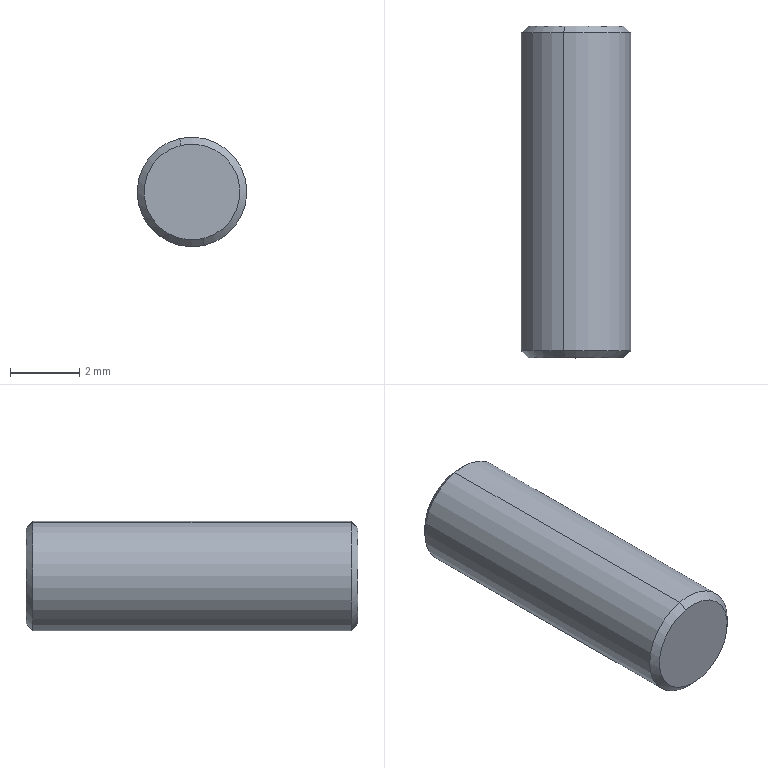Part | STEP file | 4-20.sldasm-Part-227 | 1 solid | 8 faces | box 3.175 x 9.6 x 3.175 mm | volume 75.624 mm3 | cone 4 | cylinder 2 | plane 2 | commonest cylinder face diameters 3.175 x2
STEP:
#1=CARTESIAN_POINT('',(146.186,602.225,-119.7));
#2=VERTEX_POINT('',#1);
#3=CARTESIAN_POINT('',(145.562,602.225,-116.996));
#4=VERTEX_POINT('',#3);
#5=CARTESIAN_POINT('',(145.874,602.225,-118.348));
#6=DIRECTION('',(0.,-1.,0.));
#7=DIRECTION('',(-0.225,0.,0.9744));
#8=AXIS2_PLACEMENT_3D('',#5,#6,#7);
#9=CIRCLE('',#8,1.387);
#10=EDGE_CURVE('',#2,#4,#9,.T.);
#11=ORIENTED_EDGE('',*,*,#10,.T.);
#12=CARTESIAN_POINT('',(145.517,602.025,-116.801));
#13=VERTEX_POINT('',#12);
#14=CARTESIAN_POINT('',(145.562,602.225,-116.996));
#15=DIRECTION('',(-0.1591,-0.7071,0.689));
#16=VECTOR('',#15,1000.);
#17=LINE('',#14,#16);
#18=EDGE_CURVE('',#4,#13,#17,.T.);
#19=ORIENTED_EDGE('',*,*,#18,.T.);
#20=CARTESIAN_POINT('',(146.231,602.025,-119.895));
#21=VERTEX_POINT('',#20);
#22=CARTESIAN_POINT('',(145.874,602.025,-118.348));
#23=DIRECTION('',(0.,1.,0.));
#24=DIRECTION('',(-0.225,0.,0.9744));
#25=AXIS2_PLACEMENT_3D('',#22,#23,#24);
#26=CIRCLE('',#25,1.587);
#27=EDGE_CURVE('',#13,#21,#26,.T.);
#28=ORIENTED_EDGE('',*,*,#27,.T.);
#29=CARTESIAN_POINT('',(146.186,602.225,-119.7));
#30=DIRECTION('',(0.1591,-0.7071,-0.689));
#31=VECTOR('',#30,1000.);
#32=LINE('',#29,#31);
#33=EDGE_CURVE('',#2,#21,#32,.T.);
#34=ORIENTED_EDGE('',*,*,#33,.F.);
#35=EDGE_LOOP('',(#11,#19,#28,#34));
#36=FACE_OUTER_BOUND('',#35,.T.);
#37=CARTESIAN_POINT('',(145.874,602.225,-118.348));
#38=DIRECTION('',(0.,-1.,0.));
#39=DIRECTION('',(0.225,0.,-0.9744));
#40=AXIS2_PLACEMENT_3D('',#37,#38,#39);
#41=CONICAL_SURFACE('',#40,1.387,0.7854);
#42=ADVANCED_FACE('',(#36),#41,.T.);
#43=CARTESIAN_POINT('',(145.562,592.625,-116.996));
#44=VERTEX_POINT('',#43);
#45=CARTESIAN_POINT('',(146.186,592.625,-119.7));
#46=VERTEX_POINT('',#45);
#47=CARTESIAN_POINT('',(145.874,592.625,-118.348));
#48=DIRECTION('',(0.,1.,0.));
#49=DIRECTION('',(-0.225,0.,0.9744));
#50=AXIS2_PLACEMENT_3D('',#47,#48,#49);
#51=CIRCLE('',#50,1.387);
#52=EDGE_CURVE('',#44,#46,#51,.T.);
#53=ORIENTED_EDGE('',*,*,#52,.T.);
#54=CARTESIAN_POINT('',(146.231,592.825,-119.895));
#55=VERTEX_POINT('',#54);
#56=CARTESIAN_POINT('',(146.231,592.825,-119.895));
#57=DIRECTION('',(0.1591,0.7071,-0.689));
#58=VECTOR('',#57,1000.);
#59=LINE('',#56,#58);
#60=EDGE_CURVE('',#46,#55,#59,.T.);
#61=ORIENTED_EDGE('',*,*,#60,.T.);
#62=CARTESIAN_POINT('',(145.517,592.825,-116.801));
#63=VERTEX_POINT('',#62);
#64=CARTESIAN_POINT('',(145.874,592.825,-118.348));
#65=DIRECTION('',(0.,-1.,0.));
#66=DIRECTION('',(-0.225,0.,0.9744));
#67=AXIS2_PLACEMENT_3D('',#64,#65,#66);
#68=CIRCLE('',#67,1.587);
#69=EDGE_CURVE('',#55,#63,#68,.T.);
#70=ORIENTED_EDGE('',*,*,#69,.T.);
#71=CARTESIAN_POINT('',(145.517,592.825,-116.801));
#72=DIRECTION('',(-0.1591,0.7071,0.689));
#73=VECTOR('',#72,1000.);
#74=LINE('',#71,#73);
#75=EDGE_CURVE('',#44,#63,#74,.T.);
#76=ORIENTED_EDGE('',*,*,#75,.F.);
#77=EDGE_LOOP('',(#53,#61,#70,#76));
#78=FACE_OUTER_BOUND('',#77,.T.);
#79=CARTESIAN_POINT('',(145.874,592.825,-118.348));
#80=DIRECTION('',(0.,1.,0.));
#81=DIRECTION('',(-0.225,0.,0.9744));
#82=AXIS2_PLACEMENT_3D('',#79,#80,#81);
#83=CONICAL_SURFACE('',#82,1.587,0.7854);
#84=ADVANCED_FACE('',(#78),#83,.T.);
#85=ORIENTED_EDGE('',*,*,#27,.F.);
#86=CARTESIAN_POINT('',(145.517,602.425,-116.801));
#87=DIRECTION('',(0.,-1.,0.));
#88=VECTOR('',#87,1000.);
#89=LINE('',#86,#88);
#90=EDGE_CURVE('',#13,#63,#89,.T.);
#91=ORIENTED_EDGE('',*,*,#90,.T.);
#92=ORIENTED_EDGE('',*,*,#69,.F.);
#93=CARTESIAN_POINT('',(146.231,602.425,-119.895));
#94=DIRECTION('',(0.,-1.,0.));
#95=VECTOR('',#94,1000.);
#96=LINE('',#93,#95);
#97=EDGE_CURVE('',#21,#55,#96,.T.);
#98=ORIENTED_EDGE('',*,*,#97,.F.);
#99=EDGE_LOOP('',(#85,#91,#92,#98));
#100=FACE_OUTER_BOUND('',#99,.T.);
#101=CARTESIAN_POINT('',(145.874,602.425,-118.348));
#102=DIRECTION('',(0.,-1.,0.));
#103=DIRECTION('',(0.225,0.,-0.9744));
#104=AXIS2_PLACEMENT_3D('',#101,#102,#103);
#105=CYLINDRICAL_SURFACE('',#104,1.587);
#106=ADVANCED_FACE('',(#100),#105,.T.);
#107=ORIENTED_EDGE('',*,*,#90,.F.);
#108=CARTESIAN_POINT('',(145.874,602.025,-118.348));
#109=DIRECTION('',(0.,1.,0.));
#110=DIRECTION('',(-0.225,0.,0.9744));
#111=AXIS2_PLACEMENT_3D('',#108,#109,#110);
#112=CIRCLE('',#111,1.588);
#113=EDGE_CURVE('',#21,#13,#112,.T.);
#114=ORIENTED_EDGE('',*,*,#113,.F.);
#115=ORIENTED_EDGE('',*,*,#97,.T.);
#116=CARTESIAN_POINT('',(145.874,592.825,-118.348));
#117=DIRECTION('',(0.,-1.,0.));
#118=DIRECTION('',(-0.225,0.,0.9744));
#119=AXIS2_PLACEMENT_3D('',#116,#117,#118);
#120=CIRCLE('',#119,1.587);
#121=EDGE_CURVE('',#63,#55,#120,.T.);
#122=ORIENTED_EDGE('',*,*,#121,.F.);
#123=EDGE_LOOP('',(#107,#114,#115,#122));
#124=FACE_OUTER_BOUND('',#123,.T.);
#125=CARTESIAN_POINT('',(145.874,602.425,-118.348));
#126=DIRECTION('',(0.,-1.,0.));
#127=DIRECTION('',(0.225,0.,-0.9744));
#128=AXIS2_PLACEMENT_3D('',#125,#126,#127);
#129=CYLINDRICAL_SURFACE('',#128,1.587);
#130=ADVANCED_FACE('',(#124),#129,.T.);
#131=ORIENTED_EDGE('',*,*,#10,.F.);
#132=CARTESIAN_POINT('',(145.874,602.225,-118.348));
#133=DIRECTION('',(0.,-1.,0.));
#134=DIRECTION('',(-0.225,0.,0.9744));
#135=AXIS2_PLACEMENT_3D('',#132,#133,#134);
#136=CIRCLE('',#135,1.387);
#137=EDGE_CURVE('',#4,#2,#136,.T.);
#138=ORIENTED_EDGE('',*,*,#137,.F.);
#139=EDGE_LOOP('',(#131,#138));
#140=FACE_OUTER_BOUND('',#139,.T.);
#141=CARTESIAN_POINT('',(145.874,602.225,-118.348));
#142=DIRECTION('',(0.,1.,0.));
#143=DIRECTION('',(-0.225,0.,0.9744));
#144=AXIS2_PLACEMENT_3D('',#141,#142,#143);
#145=PLANE('',#144);
#146=ADVANCED_FACE('',(#140),#145,.T.);
#147=ORIENTED_EDGE('',*,*,#52,.F.);
#148=CARTESIAN_POINT('',(145.874,592.625,-118.348));
#149=DIRECTION('',(0.,1.,0.));
#150=DIRECTION('',(-0.225,0.,0.9744));
#151=AXIS2_PLACEMENT_3D('',#148,#149,#150);
#152=CIRCLE('',#151,1.387);
#153=EDGE_CURVE('',#46,#44,#152,.T.);
#154=ORIENTED_EDGE('',*,*,#153,.F.);
#155=EDGE_LOOP('',(#147,#154));
#156=FACE_OUTER_BOUND('',#155,.T.);
#157=CARTESIAN_POINT('',(145.874,592.625,-118.348));
#158=DIRECTION('',(0.,1.,0.));
#159=DIRECTION('',(-0.225,0.,0.9744));
#160=AXIS2_PLACEMENT_3D('',#157,#158,#159);
#161=PLANE('',#160);
#162=ADVANCED_FACE('',(#156),#161,.F.);
#163=ORIENTED_EDGE('',*,*,#60,.F.);
#164=ORIENTED_EDGE('',*,*,#153,.T.);
#165=ORIENTED_EDGE('',*,*,#75,.T.);
#166=ORIENTED_EDGE('',*,*,#121,.T.);
#167=EDGE_LOOP('',(#163,#164,#165,#166));
#168=FACE_OUTER_BOUND('',#167,.T.);
#169=CARTESIAN_POINT('',(145.874,592.825,-118.348));
#170=DIRECTION('',(0.,1.,0.));
#171=DIRECTION('',(-0.225,0.,0.9744));
#172=AXIS2_PLACEMENT_3D('',#169,#170,#171);
#173=CONICAL_SURFACE('',#172,1.587,0.7854);
#174=ADVANCED_FACE('',(#168),#173,.T.);
#175=ORIENTED_EDGE('',*,*,#18,.F.);
#176=ORIENTED_EDGE('',*,*,#137,.T.);
#177=ORIENTED_EDGE('',*,*,#33,.T.);
#178=ORIENTED_EDGE('',*,*,#113,.T.);
#179=EDGE_LOOP('',(#175,#176,#177,#178));
#180=FACE_OUTER_BOUND('',#179,.T.);
#181=CARTESIAN_POINT('',(145.874,602.225,-118.348));
#182=DIRECTION('',(0.,-1.,0.));
#183=DIRECTION('',(0.225,0.,-0.9744));
#184=AXIS2_PLACEMENT_3D('',#181,#182,#183);
#185=CONICAL_SURFACE('',#184,1.387,0.7854);
#186=ADVANCED_FACE('',(#180),#185,.T.);
#187=CLOSED_SHELL('',(#42,#84,#106,#130,#146,#162,#174,#186));
#188=MANIFOLD_SOLID_BREP('',#187);
#189=CARTESIAN_POINT('',(0.,0.,0.));
#190=DIRECTION('',(0.,0.,1.));
#191=DIRECTION('',(1.,0.,0.));
#192=AXIS2_PLACEMENT_3D('',#189,#190,#191);
#193=(LENGTH_UNIT()NAMED_UNIT(*)SI_UNIT(.MILLI.,.METRE.));
#194=UNCERTAINTY_MEASURE_WITH_UNIT(LENGTH_MEASURE(0.00001),#193,'','');
#195=(NAMED_UNIT(*)PLANE_ANGLE_UNIT()SI_UNIT($,.RADIAN.));
#196=(NAMED_UNIT(*)SI_UNIT($,.STERADIAN.)SOLID_ANGLE_UNIT());
#197=(GEOMETRIC_REPRESENTATION_CONTEXT(3)GLOBAL_UNCERTAINTY_ASSIGNED_CONTEXT((#194))GLOBAL_UNIT_ASSIGNED_CONTEXT((#193,#195,#196))REPRESENTATION_CONTEXT('',''));
#198=ADVANCED_BREP_SHAPE_REPRESENTATION('',(#188,#192),#197);